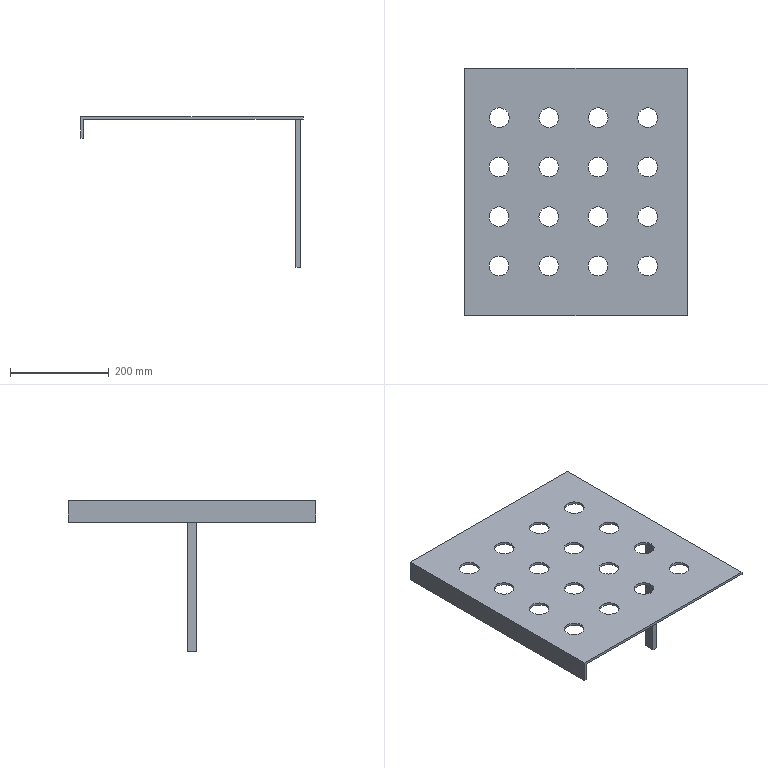Part | SolidWorks | features ICE 3, BaseBody 2 | 1 solid | 45 faces | box 450 x 500 x 305 mm | volume 1181124 mm3 | cylinder 32 | plane 13 | commonest cylinder face diameters 40 x32
STEP:
#1=CARTESIAN_POINT('',(155.,182.201,23.249));
#2=VERTEX_POINT('',#1);
#3=CARTESIAN_POINT('',(195.,182.201,23.249));
#4=VERTEX_POINT('',#3);
#5=CARTESIAN_POINT('',(175.,182.201,23.249));
#6=DIRECTION('',(0.,0.,1.));
#7=DIRECTION('',(1.,0.,0.));
#8=AXIS2_PLACEMENT_3D('',#5,#6,#7);
#9=CIRCLE('',#8,20.);
#10=EDGE_CURVE('',#2,#4,#9,.T.);
#11=ORIENTED_EDGE('',*,*,#10,.F.);
#12=CARTESIAN_POINT('',(155.,182.201,28.249));
#13=VERTEX_POINT('',#12);
#14=CARTESIAN_POINT('',(155.,182.201,23.249));
#15=DIRECTION('',(0.,0.,1.));
#16=VECTOR('',#15,1000.);
#17=LINE('',#14,#16);
#18=EDGE_CURVE('',#2,#13,#17,.T.);
#19=ORIENTED_EDGE('',*,*,#18,.T.);
#20=CARTESIAN_POINT('',(195.,182.201,28.249));
#21=VERTEX_POINT('',#20);
#22=CARTESIAN_POINT('',(175.,182.201,28.249));
#23=DIRECTION('',(0.,0.,1.));
#24=DIRECTION('',(1.,0.,0.));
#25=AXIS2_PLACEMENT_3D('',#22,#23,#24);
#26=CIRCLE('',#25,20.);
#27=EDGE_CURVE('',#13,#21,#26,.T.);
#28=ORIENTED_EDGE('',*,*,#27,.T.);
#29=CARTESIAN_POINT('',(195.,182.201,23.249));
#30=DIRECTION('',(0.,0.,1.));
#31=VECTOR('',#30,1000.);
#32=LINE('',#29,#31);
#33=EDGE_CURVE('',#4,#21,#32,.T.);
#34=ORIENTED_EDGE('',*,*,#33,.F.);
#35=EDGE_LOOP('',(#11,#19,#28,#34));
#36=FACE_OUTER_BOUND('',#35,.T.);
#37=CARTESIAN_POINT('',(175.,182.201,23.249));
#38=DIRECTION('',(0.,0.,1.));
#39=DIRECTION('',(1.,0.,0.));
#40=AXIS2_PLACEMENT_3D('',#37,#38,#39);
#41=CYLINDRICAL_SURFACE('',#40,20.);
#42=ADVANCED_FACE('',(#36),#41,.F.);
#43=CARTESIAN_POINT('',(254.334,182.201,23.249));
#44=VERTEX_POINT('',#43);
#45=CARTESIAN_POINT('',(294.334,182.201,23.249));
#46=VERTEX_POINT('',#45);
#47=CARTESIAN_POINT('',(274.334,182.201,23.249));
#48=DIRECTION('',(0.,0.,1.));
#49=DIRECTION('',(1.,0.,0.));
#50=AXIS2_PLACEMENT_3D('',#47,#48,#49);
#51=CIRCLE('',#50,20.);
#52=EDGE_CURVE('',#44,#46,#51,.T.);
#53=ORIENTED_EDGE('',*,*,#52,.F.);
#54=CARTESIAN_POINT('',(254.334,182.201,28.249));
#55=VERTEX_POINT('',#54);
#56=CARTESIAN_POINT('',(254.334,182.201,23.249));
#57=DIRECTION('',(0.,0.,1.));
#58=VECTOR('',#57,1000.);
#59=LINE('',#56,#58);
#60=EDGE_CURVE('',#44,#55,#59,.T.);
#61=ORIENTED_EDGE('',*,*,#60,.T.);
#62=CARTESIAN_POINT('',(294.334,182.201,28.249));
#63=VERTEX_POINT('',#62);
#64=CARTESIAN_POINT('',(274.334,182.201,28.249));
#65=DIRECTION('',(0.,0.,1.));
#66=DIRECTION('',(1.,0.,0.));
#67=AXIS2_PLACEMENT_3D('',#64,#65,#66);
#68=CIRCLE('',#67,20.);
#69=EDGE_CURVE('',#55,#63,#68,.T.);
#70=ORIENTED_EDGE('',*,*,#69,.T.);
#71=CARTESIAN_POINT('',(294.334,182.201,23.249));
#72=DIRECTION('',(0.,0.,1.));
#73=VECTOR('',#72,1000.);
#74=LINE('',#71,#73);
#75=EDGE_CURVE('',#46,#63,#74,.T.);
#76=ORIENTED_EDGE('',*,*,#75,.F.);
#77=EDGE_LOOP('',(#53,#61,#70,#76));
#78=FACE_OUTER_BOUND('',#77,.T.);
#79=CARTESIAN_POINT('',(274.334,182.201,23.249));
#80=DIRECTION('',(0.,0.,1.));
#81=DIRECTION('',(1.,0.,0.));
#82=AXIS2_PLACEMENT_3D('',#79,#80,#81);
#83=CYLINDRICAL_SURFACE('',#82,20.);
#84=ADVANCED_FACE('',(#78),#83,.F.);
#85=CARTESIAN_POINT('',(355.,182.201,23.249));
#86=VERTEX_POINT('',#85);
#87=CARTESIAN_POINT('',(395.,182.201,23.249));
#88=VERTEX_POINT('',#87);
#89=CARTESIAN_POINT('',(375.,182.201,23.249));
#90=DIRECTION('',(0.,0.,1.));
#91=DIRECTION('',(1.,0.,0.));
#92=AXIS2_PLACEMENT_3D('',#89,#90,#91);
#93=CIRCLE('',#92,20.);
#94=EDGE_CURVE('',#86,#88,#93,.T.);
#95=ORIENTED_EDGE('',*,*,#94,.F.);
#96=CARTESIAN_POINT('',(355.,182.201,28.249));
#97=VERTEX_POINT('',#96);
#98=CARTESIAN_POINT('',(355.,182.201,23.249));
#99=DIRECTION('',(0.,0.,1.));
#100=VECTOR('',#99,1000.);
#101=LINE('',#98,#100);
#102=EDGE_CURVE('',#86,#97,#101,.T.);
#103=ORIENTED_EDGE('',*,*,#102,.T.);
#104=CARTESIAN_POINT('',(395.,182.201,28.249));
#105=VERTEX_POINT('',#104);
#106=CARTESIAN_POINT('',(375.,182.201,28.249));
#107=DIRECTION('',(0.,0.,1.));
#108=DIRECTION('',(1.,0.,0.));
#109=AXIS2_PLACEMENT_3D('',#106,#107,#108);
#110=CIRCLE('',#109,20.);
#111=EDGE_CURVE('',#97,#105,#110,.T.);
#112=ORIENTED_EDGE('',*,*,#111,.T.);
#113=CARTESIAN_POINT('',(395.,182.201,23.249));
#114=DIRECTION('',(0.,0.,1.));
#115=VECTOR('',#114,1000.);
#116=LINE('',#113,#115);
#117=EDGE_CURVE('',#88,#105,#116,.T.);
#118=ORIENTED_EDGE('',*,*,#117,.F.);
#119=EDGE_LOOP('',(#95,#103,#112,#118));
#120=FACE_OUTER_BOUND('',#119,.T.);
#121=CARTESIAN_POINT('',(375.,182.201,23.249));
#122=DIRECTION('',(0.,0.,1.));
#123=DIRECTION('',(1.,0.,0.));
#124=AXIS2_PLACEMENT_3D('',#121,#122,#123);
#125=CYLINDRICAL_SURFACE('',#124,20.);
#126=ADVANCED_FACE('',(#120),#125,.F.);
#127=CARTESIAN_POINT('',(54.334,81.955,23.249));
#128=VERTEX_POINT('',#127);
#129=CARTESIAN_POINT('',(94.334,81.955,23.249));
#130=VERTEX_POINT('',#129);
#131=CARTESIAN_POINT('',(74.334,81.955,23.249));
#132=DIRECTION('',(0.,0.,1.));
#133=DIRECTION('',(1.,0.,0.));
#134=AXIS2_PLACEMENT_3D('',#131,#132,#133);
#135=CIRCLE('',#134,20.);
#136=EDGE_CURVE('',#128,#130,#135,.T.);
#137=ORIENTED_EDGE('',*,*,#136,.F.);
#138=CARTESIAN_POINT('',(54.334,81.955,28.249));
#139=VERTEX_POINT('',#138);
#140=CARTESIAN_POINT('',(54.334,81.955,23.249));
#141=DIRECTION('',(0.,0.,1.));
#142=VECTOR('',#141,1000.);
#143=LINE('',#140,#142);
#144=EDGE_CURVE('',#128,#139,#143,.T.);
#145=ORIENTED_EDGE('',*,*,#144,.T.);
#146=CARTESIAN_POINT('',(94.334,81.955,28.249));
#147=VERTEX_POINT('',#146);
#148=CARTESIAN_POINT('',(74.334,81.955,28.249));
#149=DIRECTION('',(0.,0.,1.));
#150=DIRECTION('',(1.,0.,0.));
#151=AXIS2_PLACEMENT_3D('',#148,#149,#150);
#152=CIRCLE('',#151,20.);
#153=EDGE_CURVE('',#139,#147,#152,.T.);
#154=ORIENTED_EDGE('',*,*,#153,.T.);
#155=CARTESIAN_POINT('',(94.334,81.955,23.249));
#156=DIRECTION('',(0.,0.,1.));
#157=VECTOR('',#156,1000.);
#158=LINE('',#155,#157);
#159=EDGE_CURVE('',#130,#147,#158,.T.);
#160=ORIENTED_EDGE('',*,*,#159,.F.);
#161=EDGE_LOOP('',(#137,#145,#154,#160));
#162=FACE_OUTER_BOUND('',#161,.T.);
#163=CARTESIAN_POINT('',(74.334,81.955,23.249));
#164=DIRECTION('',(0.,0.,1.));
#165=DIRECTION('',(1.,0.,0.));
#166=AXIS2_PLACEMENT_3D('',#163,#164,#165);
#167=CYLINDRICAL_SURFACE('',#166,20.);
#168=ADVANCED_FACE('',(#162),#167,.F.);
#169=CARTESIAN_POINT('',(155.,282.201,23.249));
#170=VERTEX_POINT('',#169);
#171=CARTESIAN_POINT('',(195.,282.201,23.249));
#172=VERTEX_POINT('',#171);
#173=CARTESIAN_POINT('',(175.,282.201,23.249));
#174=DIRECTION('',(0.,0.,1.));
#175=DIRECTION('',(1.,0.,0.));
#176=AXIS2_PLACEMENT_3D('',#173,#174,#175);
#177=CIRCLE('',#176,20.);
#178=EDGE_CURVE('',#170,#172,#177,.T.);
#179=ORIENTED_EDGE('',*,*,#178,.F.);
#180=CARTESIAN_POINT('',(155.,282.201,28.249));
#181=VERTEX_POINT('',#180);
#182=CARTESIAN_POINT('',(155.,282.201,23.249));
#183=DIRECTION('',(0.,0.,1.));
#184=VECTOR('',#183,1000.);
#185=LINE('',#182,#184);
#186=EDGE_CURVE('',#170,#181,#185,.T.);
#187=ORIENTED_EDGE('',*,*,#186,.T.);
#188=CARTESIAN_POINT('',(195.,282.201,28.249));
#189=VERTEX_POINT('',#188);
#190=CARTESIAN_POINT('',(175.,282.201,28.249));
#191=DIRECTION('',(0.,0.,1.));
#192=DIRECTION('',(1.,0.,0.));
#193=AXIS2_PLACEMENT_3D('',#190,#191,#192);
#194=CIRCLE('',#193,20.);
#195=EDGE_CURVE('',#181,#189,#194,.T.);
#196=ORIENTED_EDGE('',*,*,#195,.T.);
#197=CARTESIAN_POINT('',(195.,282.201,23.249));
#198=DIRECTION('',(0.,0.,1.));
#199=VECTOR('',#198,1000.);
#200=LINE('',#197,#199);
#201=EDGE_CURVE('',#172,#189,#200,.T.);
#202=ORIENTED_EDGE('',*,*,#201,.F.);
#203=EDGE_LOOP('',(#179,#187,#196,#202));
#204=FACE_OUTER_BOUND('',#203,.T.);
#205=CARTESIAN_POINT('',(175.,282.201,23.249));
#206=DIRECTION('',(0.,0.,1.));
#207=DIRECTION('',(1.,0.,0.));
#208=AXIS2_PLACEMENT_3D('',#205,#206,#207);
#209=CYLINDRICAL_SURFACE('',#208,20.);
#210=ADVANCED_FACE('',(#204),#209,.F.);
#211=CARTESIAN_POINT('',(255.,282.201,23.249));
#212=VERTEX_POINT('',#211);
#213=CARTESIAN_POINT('',(295.,282.201,23.249));
#214=VERTEX_POINT('',#213);
#215=CARTESIAN_POINT('',(275.,282.201,23.249));
#216=DIRECTION('',(0.,0.,1.));
#217=DIRECTION('',(1.,0.,0.));
#218=AXIS2_PLACEMENT_3D('',#215,#216,#217);
#219=CIRCLE('',#218,20.);
#220=EDGE_CURVE('',#212,#214,#219,.T.);
#221=ORIENTED_EDGE('',*,*,#220,.F.);
#222=CARTESIAN_POINT('',(255.,282.201,28.249));
#223=VERTEX_POINT('',#222);
#224=CARTESIAN_POINT('',(255.,282.201,23.249));
#225=DIRECTION('',(0.,0.,1.));
#226=VECTOR('',#225,1000.);
#227=LINE('',#224,#226);
#228=EDGE_CURVE('',#212,#223,#227,.T.);
#229=ORIENTED_EDGE('',*,*,#228,.T.);
#230=CARTESIAN_POINT('',(295.,282.201,28.249));
#231=VERTEX_POINT('',#230);
#232=CARTESIAN_POINT('',(275.,282.201,28.249));
#233=DIRECTION('',(0.,0.,1.));
#234=DIRECTION('',(1.,0.,0.));
#235=AXIS2_PLACEMENT_3D('',#232,#233,#234);
#236=CIRCLE('',#235,20.);
#237=EDGE_CURVE('',#223,#231,#236,.T.);
#238=ORIENTED_EDGE('',*,*,#237,.T.);
#239=CARTESIAN_POINT('',(295.,282.201,23.249));
#240=DIRECTION('',(0.,0.,1.));
#241=VECTOR('',#240,1000.);
#242=LINE('',#239,#241);
#243=EDGE_CURVE('',#214,#231,#242,.T.);
#244=ORIENTED_EDGE('',*,*,#243,.F.);
#245=EDGE_LOOP('',(#221,#229,#238,#244));
#246=FACE_OUTER_BOUND('',#245,.T.);
#247=CARTESIAN_POINT('',(275.,282.201,23.249));
#248=DIRECTION('',(0.,0.,1.));
#249=DIRECTION('',(1.,0.,0.));
#250=AXIS2_PLACEMENT_3D('',#247,#248,#249);
#251=CYLINDRICAL_SURFACE('',#250,20.);
#252=ADVANCED_FACE('',(#246),#251,.F.);
#253=CARTESIAN_POINT('',(355.,282.201,23.249));
#254=VERTEX_POINT('',#253);
#255=CARTESIAN_POINT('',(395.,282.201,23.249));
#256=VERTEX_POINT('',#255);
#257=CARTESIAN_POINT('',(375.,282.201,23.249));
#258=DIRECTION('',(0.,0.,1.));
#259=DIRECTION('',(1.,0.,0.));
#260=AXIS2_PLACEMENT_3D('',#257,#258,#259);
#261=CIRCLE('',#260,20.);
#262=EDGE_CURVE('',#254,#256,#261,.T.);
#263=ORIENTED_EDGE('',*,*,#262,.F.);
#264=CARTESIAN_POINT('',(355.,282.201,28.249));
#265=VERTEX_POINT('',#264);
#266=CARTESIAN_POINT('',(355.,282.201,23.249));
#267=DIRECTION('',(0.,0.,1.));
#268=VECTOR('',#267,1000.);
#269=LINE('',#266,#268);
#270=EDGE_CURVE('',#254,#265,#269,.T.);
#271=ORIENTED_EDGE('',*,*,#270,.T.);
#272=CARTESIAN_POINT('',(395.,282.201,28.249));
#273=VERTEX_POINT('',#272);
#274=CARTESIAN_POINT('',(375.,282.201,28.249));
#275=DIRECTION('',(0.,0.,1.));
#276=DIRECTION('',(1.,0.,0.));
#277=AXIS2_PLACEMENT_3D('',#274,#275,#276);
#278=CIRCLE('',#277,20.);
#279=EDGE_CURVE('',#265,#273,#278,.T.);
#280=ORIENTED_EDGE('',*,*,#279,.T.);
#281=CARTESIAN_POINT('',(395.,282.201,23.249));
#282=DIRECTION('',(0.,0.,1.));
#283=VECTOR('',#282,1000.);
#284=LINE('',#281,#283);
#285=EDGE_CURVE('',#256,#273,#284,.T.);
#286=ORIENTED_EDGE('',*,*,#285,.F.);
#287=EDGE_LOOP('',(#263,#271,#280,#286));
#288=FACE_OUTER_BOUND('',#287,.T.);
#289=CARTESIAN_POINT('',(375.,282.201,23.249));
#290=DIRECTION('',(0.,0.,1.));
#291=DIRECTION('',(1.,0.,0.));
#292=AXIS2_PLACEMENT_3D('',#289,#290,#291);
#293=CYLINDRICAL_SURFACE('',#292,20.);
#294=ADVANCED_FACE('',(#288),#293,.F.);
#295=CARTESIAN_POINT('',(54.334,182.201,23.249));
#296=VERTEX_POINT('',#295);
#297=CARTESIAN_POINT('',(94.334,182.201,23.249));
#298=VERTEX_POINT('',#297);
#299=CARTESIAN_POINT('',(74.334,182.201,23.249));
#300=DIRECTION('',(0.,0.,1.));
#301=DIRECTION('',(1.,0.,0.));
#302=AXIS2_PLACEMENT_3D('',#299,#300,#301);
#303=CIRCLE('',#302,20.);
#304=EDGE_CURVE('',#296,#298,#303,.T.);
#305=ORIENTED_EDGE('',*,*,#304,.F.);
#306=CARTESIAN_POINT('',(54.334,182.201,28.249));
#307=VERTEX_POINT('',#306);
#308=CARTESIAN_POINT('',(54.334,182.201,23.249));
#309=DIRECTION('',(0.,0.,1.));
#310=VECTOR('',#309,1000.);
#311=LINE('',#308,#310);
#312=EDGE_CURVE('',#296,#307,#311,.T.);
#313=ORIENTED_EDGE('',*,*,#312,.T.);
#314=CARTESIAN_POINT('',(94.334,182.201,28.249));
#315=VERTEX_POINT('',#314);
#316=CARTESIAN_POINT('',(74.334,182.201,28.249));
#317=DIRECTION('',(0.,0.,1.));
#318=DIRECTION('',(1.,0.,0.));
#319=AXIS2_PLACEMENT_3D('',#316,#317,#318);
#320=CIRCLE('',#319,20.);
#321=EDGE_CURVE('',#307,#315,#320,.T.);
#322=ORIENTED_EDGE('',*,*,#321,.T.);
#323=CARTESIAN_POINT('',(94.334,182.201,23.249));
#324=DIRECTION('',(0.,0.,1.));
#325=VECTOR('',#324,1000.);
#326=LINE('',#323,#325);
#327=EDGE_CURVE('',#298,#315,#326,.T.);
#328=ORIENTED_EDGE('',*,*,#327,.F.);
#329=EDGE_LOOP('',(#305,#313,#322,#328));
#330=FACE_OUTER_BOUND('',#329,.T.);
#331=CARTESIAN_POINT('',(74.334,182.201,23.249));
#332=DIRECTION('',(0.,0.,1.));
#333=DIRECTION('',(1.,0.,0.));
#334=AXIS2_PLACEMENT_3D('',#331,#332,#333);
#335=CYLINDRICAL_SURFACE('',#334,20.);
#336=ADVANCED_FACE('',(#330),#335,.F.);
#337=CARTESIAN_POINT('',(355.,-18.045,23.249));
#338=VERTEX_POINT('',#337);
#339=CARTESIAN_POINT('',(395.,-18.045,23.249));
#340=VERTEX_POINT('',#339);
#341=CARTESIAN_POINT('',(375.,-18.045,23.249));
#342=DIRECTION('',(0.,0.,1.));
#343=DIRECTION('',(1.,0.,0.));
#344=AXIS2_PLACEMENT_3D('',#341,#342,#343);
#345=CIRCLE('',#344,20.);
#346=EDGE_CURVE('',#338,#340,#345,.T.);
#347=ORIENTED_EDGE('',*,*,#346,.F.);
#348=CARTESIAN_POINT('',(355.,-18.045,28.249));
#349=VERTEX_POINT('',#348);
#350=CARTESIAN_POINT('',(355.,-18.045,23.249));
#351=DIRECTION('',(0.,0.,1.));
#352=VECTOR('',#351,1000.);
#353=LINE('',#350,#352);
#354=EDGE_CURVE('',#338,#349,#353,.T.);
#355=ORIENTED_EDGE('',*,*,#354,.T.);
#356=CARTESIAN_POINT('',(395.,-18.045,28.249));
#357=VERTEX_POINT('',#356);
#358=CARTESIAN_POINT('',(375.,-18.045,28.249));
#359=DIRECTION('',(0.,0.,1.));
#360=DIRECTION('',(1.,0.,0.));
#361=AXIS2_PLACEMENT_3D('',#358,#359,#360);
#362=CIRCLE('',#361,20.);
#363=EDGE_CURVE('',#349,#357,#362,.T.);
#364=ORIENTED_EDGE('',*,*,#363,.T.);
#365=CARTESIAN_POINT('',(395.,-18.045,23.249));
#366=DIRECTION('',(0.,0.,1.));
#367=VECTOR('',#366,1000.);
#368=LINE('',#365,#367);
#369=EDGE_CURVE('',#340,#357,#368,.T.);
#370=ORIENTED_EDGE('',*,*,#369,.F.);
#371=EDGE_LOOP('',(#347,#355,#364,#370));
#372=FACE_OUTER_BOUND('',#371,.T.);
#373=CARTESIAN_POINT('',(375.,-18.045,23.249));
#374=DIRECTION('',(0.,0.,1.));
#375=DIRECTION('',(1.,0.,0.));
#376=AXIS2_PLACEMENT_3D('',#373,#374,#375);
#377=CYLINDRICAL_SURFACE('',#376,20.);
#378=ADVANCED_FACE('',(#372),#377,.F.);
#379=CARTESIAN_POINT('',(254.334,-18.045,23.249));
#380=VERTEX_POINT('',#379);
#381=CARTESIAN_POINT('',(294.334,-18.045,23.249));
#382=VERTEX_POINT('',#381);
#383=CARTESIAN_POINT('',(274.334,-18.045,23.249));
#384=DIRECTION('',(0.,0.,1.));
#385=DIRECTION('',(1.,0.,0.));
#386=AXIS2_PLACEMENT_3D('',#383,#384,#385);
#387=CIRCLE('',#386,20.);
#388=EDGE_CURVE('',#380,#382,#387,.T.);
#389=ORIENTED_EDGE('',*,*,#388,.F.);
#390=CARTESIAN_POINT('',(254.334,-18.045,28.249));
#391=VERTEX_POINT('',#390);
#392=CARTESIAN_POINT('',(254.334,-18.045,23.249));
#393=DIRECTION('',(0.,0.,1.));
#394=VECTOR('',#393,1000.);
#395=LINE('',#392,#394);
#396=EDGE_CURVE('',#380,#391,#395,.T.);
#397=ORIENTED_EDGE('',*,*,#396,.T.);
#398=CARTESIAN_POINT('',(294.334,-18.045,28.249));
#399=VERTEX_POINT('',#398);
#400=CARTESIAN_POINT('',(274.334,-18.045,28.249));
#401=DIRECTION('',(0.,0.,1.));
#402=DIRECTION('',(1.,0.,0.));
#403=AXIS2_PLACEMENT_3D('',#400,#401,#402);
#404=CIRCLE('',#403,20.);
#405=EDGE_CURVE('',#391,#399,#404,.T.);
#406=ORIENTED_EDGE('',*,*,#405,.T.);
#407=CARTESIAN_POINT('',(294.334,-18.045,23.249));
#408=DIRECTION('',(0.,0.,1.));
#409=VECTOR('',#408,1000.);
#410=LINE('',#407,#409);
#411=EDGE_CURVE('',#382,#399,#410,.T.);
#412=ORIENTED_EDGE('',*,*,#411,.F.);
#413=EDGE_LOOP('',(#389,#397,#406,#412));
#414=FACE_OUTER_BOUND('',#413,.T.);
#415=CARTESIAN_POINT('',(274.334,-18.045,23.249));
#416=DIRECTION('',(0.,0.,1.));
#417=DIRECTION('',(1.,0.,0.));
#418=AXIS2_PLACEMENT_3D('',#415,#416,#417);
#419=CYLINDRICAL_SURFACE('',#418,20.);
#420=ADVANCED_FACE('',(#414),#419,.F.);
#421=CARTESIAN_POINT('',(155.,-18.045,23.249));
#422=VERTEX_POINT('',#421);
#423=CARTESIAN_POINT('',(195.,-18.045,23.249));
#424=VERTEX_POINT('',#423);
#425=CARTESIAN_POINT('',(175.,-18.045,23.249));
#426=DIRECTION('',(0.,0.,1.));
#427=DIRECTION('',(1.,0.,0.));
#428=AXIS2_PLACEMENT_3D('',#425,#426,#427);
#429=CIRCLE('',#428,20.);
#430=EDGE_CURVE('',#422,#424,#429,.T.);
#431=ORIENTED_EDGE('',*,*,#430,.F.);
#432=CARTESIAN_POINT('',(155.,-18.045,28.249));
#433=VERTEX_POINT('',#432);
#434=CARTESIAN_POINT('',(155.,-18.045,23.249));
#435=DIRECTION('',(0.,0.,1.));
#436=VECTOR('',#435,1000.);
#437=LINE('',#434,#436);
#438=EDGE_CURVE('',#422,#433,#437,.T.);
#439=ORIENTED_EDGE('',*,*,#438,.T.);
#440=CARTESIAN_POINT('',(195.,-18.045,28.249));
#441=VERTEX_POINT('',#440);
#442=CARTESIAN_POINT('',(175.,-18.045,28.249));
#443=DIRECTION('',(0.,0.,1.));
#444=DIRECTION('',(1.,0.,0.));
#445=AXIS2_PLACEMENT_3D('',#442,#443,#444);
#446=CIRCLE('',#445,20.);
#447=EDGE_CURVE('',#433,#441,#446,.T.);
#448=ORIENTED_EDGE('',*,*,#447,.T.);
#449=CARTESIAN_POINT('',(195.,-18.045,23.249));
#450=DIRECTION('',(0.,0.,1.));
#451=VECTOR('',#450,1000.);
#452=LINE('',#449,#451);
#453=EDGE_CURVE('',#424,#441,#452,.T.);
#454=ORIENTED_EDGE('',*,*,#453,.F.);
#455=EDGE_LOOP('',(#431,#439,#448,#454));
#456=FACE_OUTER_BOUND('',#455,.T.);
#457=CARTESIAN_POINT('',(175.,-18.045,23.249));
#458=DIRECTION('',(0.,0.,1.));
#459=DIRECTION('',(1.,0.,0.));
#460=AXIS2_PLACEMENT_3D('',#457,#458,#459);
#461=CYLINDRICAL_SURFACE('',#460,20.);
#462=ADVANCED_FACE('',(#456),#461,.F.);
#463=CARTESIAN_POINT('',(155.,81.955,23.249));
#464=VERTEX_POINT('',#463);
#465=CARTESIAN_POINT('',(195.,81.955,23.249));
#466=VERTEX_POINT('',#465);
#467=CARTESIAN_POINT('',(175.,81.955,23.249));
#468=DIRECTION('',(0.,0.,1.));
#469=DIRECTION('',(1.,0.,0.));
#470=AXIS2_PLACEMENT_3D('',#467,#468,#469);
#471=CIRCLE('',#470,20.);
#472=EDGE_CURVE('',#464,#466,#471,.T.);
#473=ORIENTED_EDGE('',*,*,#472,.F.);
#474=CARTESIAN_POINT('',(155.,81.955,28.249));
#475=VERTEX_POINT('',#474);
#476=CARTESIAN_POINT('',(155.,81.955,23.249));
#477=DIRECTION('',(0.,0.,1.));
#478=VECTOR('',#477,1000.);
#479=LINE('',#476,#478);
#480=EDGE_CURVE('',#464,#475,#479,.T.);
#481=ORIENTED_EDGE('',*,*,#480,.T.);
#482=CARTESIAN_POINT('',(195.,81.955,28.249));
#483=VERTEX_POINT('',#482);
#484=CARTESIAN_POINT('',(175.,81.955,28.249));
#485=DIRECTION('',(0.,0.,1.));
#486=DIRECTION('',(1.,0.,0.));
#487=AXIS2_PLACEMENT_3D('',#484,#485,#486);
#488=CIRCLE('',#487,20.);
#489=EDGE_CURVE('',#475,#483,#488,.T.);
#490=ORIENTED_EDGE('',*,*,#489,.T.);
#491=CARTESIAN_POINT('',(195.,81.955,23.249));
#492=DIRECTION('',(0.,0.,1.));
#493=VECTOR('',#492,1000.);
#494=LINE('',#491,#493);
#495=EDGE_CURVE('',#466,#483,#494,.T.);
#496=ORIENTED_EDGE('',*,*,#495,.F.);
#497=EDGE_LOOP('',(#473,#481,#490,#496));
#498=FACE_OUTER_BOUND('',#497,.T.);
#499=CARTESIAN_POINT('',(175.,81.955,23.249));
#500=DIRECTION('',(0.,0.,1.));
#501=DIRECTION('',(1.,0.,0.));
#502=AXIS2_PLACEMENT_3D('',#499,#500,#501);
#503=CYLINDRICAL_SURFACE('',#502,20.);
#504=ADVANCED_FACE('',(#498),#503,.F.);
#505=CARTESIAN_POINT('',(254.334,81.955,23.249));
#506=VERTEX_POINT('',#505);
#507=CARTESIAN_POINT('',(294.334,81.955,23.249));
#508=VERTEX_POINT('',#507);
#509=CARTESIAN_POINT('',(274.334,81.955,23.249));
#510=DIRECTION('',(0.,0.,1.));
#511=DIRECTION('',(1.,0.,0.));
#512=AXIS2_PLACEMENT_3D('',#509,#510,#511);
#513=CIRCLE('',#512,20.);
#514=EDGE_CURVE('',#506,#508,#513,.T.);
#515=ORIENTED_EDGE('',*,*,#514,.F.);
#516=CARTESIAN_POINT('',(254.334,81.955,28.249));
#517=VERTEX_POINT('',#516);
#518=CARTESIAN_POINT('',(254.334,81.955,23.249));
#519=DIRECTION('',(0.,0.,1.));
#520=VECTOR('',#519,1000.);
#521=LINE('',#518,#520);
#522=EDGE_CURVE('',#506,#517,#521,.T.);
#523=ORIENTED_EDGE('',*,*,#522,.T.);
#524=CARTESIAN_POINT('',(294.334,81.955,28.249));
#525=VERTEX_POINT('',#524);
#526=CARTESIAN_POINT('',(274.334,81.955,28.249));
#527=DIRECTION('',(0.,0.,1.));
#528=DIRECTION('',(1.,0.,0.));
#529=AXIS2_PLACEMENT_3D('',#526,#527,#528);
#530=CIRCLE('',#529,20.);
#531=EDGE_CURVE('',#517,#525,#530,.T.);
#532=ORIENTED_EDGE('',*,*,#531,.T.);
#533=CARTESIAN_POINT('',(294.334,81.955,23.249));
#534=DIRECTION('',(0.,0.,1.));
#535=VECTOR('',#534,1000.);
#536=LINE('',#533,#535);
#537=EDGE_CURVE('',#508,#525,#536,.T.);
#538=ORIENTED_EDGE('',*,*,#537,.F.);
#539=EDGE_LOOP('',(#515,#523,#532,#538));
#540=FACE_OUTER_BOUND('',#539,.T.);
#541=CARTESIAN_POINT('',(274.334,81.955,23.249));
#542=DIRECTION('',(0.,0.,1.));
#543=DIRECTION('',(1.,0.,0.));
#544=AXIS2_PLACEMENT_3D('',#541,#542,#543);
#545=CYLINDRICAL_SURFACE('',#544,20.);
#546=ADVANCED_FACE('',(#540),#545,.F.);
#547=CARTESIAN_POINT('',(355.,81.955,23.249));
#548=VERTEX_POINT('',#547);
#549=CARTESIAN_POINT('',(395.,81.955,23.249));
#550=VERTEX_POINT('',#549);
#551=CARTESIAN_POINT('',(375.,81.955,23.249));
#552=DIRECTION('',(0.,0.,1.));
#553=DIRECTION('',(1.,0.,0.));
#554=AXIS2_PLACEMENT_3D('',#551,#552,#553);
#555=CIRCLE('',#554,20.);
#556=EDGE_CURVE('',#548,#550,#555,.T.);
#557=ORIENTED_EDGE('',*,*,#556,.F.);
#558=CARTESIAN_POINT('',(355.,81.955,28.249));
#559=VERTEX_POINT('',#558);
#560=CARTESIAN_POINT('',(355.,81.955,23.249));
#561=DIRECTION('',(0.,0.,1.));
#562=VECTOR('',#561,1000.);
#563=LINE('',#560,#562);
#564=EDGE_CURVE('',#548,#559,#563,.T.);
#565=ORIENTED_EDGE('',*,*,#564,.T.);
#566=CARTESIAN_POINT('',(395.,81.955,28.249));
#567=VERTEX_POINT('',#566);
#568=CARTESIAN_POINT('',(375.,81.955,28.249));
#569=DIRECTION('',(0.,0.,1.));
#570=DIRECTION('',(1.,0.,0.));
#571=AXIS2_PLACEMENT_3D('',#568,#569,#570);
#572=CIRCLE('',#571,20.);
#573=EDGE_CURVE('',#559,#567,#572,.T.);
#574=ORIENTED_EDGE('',*,*,#573,.T.);
#575=CARTESIAN_POINT('',(395.,81.955,23.249));
#576=DIRECTION('',(0.,0.,1.));
#577=VECTOR('',#576,1000.);
#578=LINE('',#575,#577);
#579=EDGE_CURVE('',#550,#567,#578,.T.);
#580=ORIENTED_EDGE('',*,*,#579,.F.);
#581=EDGE_LOOP('',(#557,#565,#574,#580));
#582=FACE_OUTER_BOUND('',#581,.T.);
#583=CARTESIAN_POINT('',(375.,81.955,23.249));
#584=DIRECTION('',(0.,0.,1.));
#585=DIRECTION('',(1.,0.,0.));
#586=AXIS2_PLACEMENT_3D('',#583,#584,#585);
#587=CYLINDRICAL_SURFACE('',#586,20.);
#588=ADVANCED_FACE('',(#582),#587,.F.);
#589=CARTESIAN_POINT('',(54.334,-18.045,23.249));
#590=VERTEX_POINT('',#589);
#591=CARTESIAN_POINT('',(94.334,-18.045,23.249));
#592=VERTEX_POINT('',#591);
#593=CARTESIAN_POINT('',(74.334,-18.045,23.249));
#594=DIRECTION('',(0.,0.,1.));
#595=DIRECTION('',(1.,0.,0.));
#596=AXIS2_PLACEMENT_3D('',#593,#594,#595);
#597=CIRCLE('',#596,20.);
#598=EDGE_CURVE('',#590,#592,#597,.T.);
#599=ORIENTED_EDGE('',*,*,#598,.F.);
#600=CARTESIAN_POINT('',(54.334,-18.045,28.249));
#601=VERTEX_POINT('',#600);
#602=CARTESIAN_POINT('',(54.334,-18.045,23.249));
#603=DIRECTION('',(0.,0.,1.));
#604=VECTOR('',#603,1000.);
#605=LINE('',#602,#604);
#606=EDGE_CURVE('',#590,#601,#605,.T.);
#607=ORIENTED_EDGE('',*,*,#606,.T.);
#608=CARTESIAN_POINT('',(94.334,-18.045,28.249));
#609=VERTEX_POINT('',#608);
#610=CARTESIAN_POINT('',(74.334,-18.045,28.249));
#611=DIRECTION('',(0.,0.,1.));
#612=DIRECTION('',(1.,0.,0.));
#613=AXIS2_PLACEMENT_3D('',#610,#611,#612);
#614=CIRCLE('',#613,20.);
#615=EDGE_CURVE('',#601,#609,#614,.T.);
#616=ORIENTED_EDGE('',*,*,#615,.T.);
#617=CARTESIAN_POINT('',(94.334,-18.045,23.249));
#618=DIRECTION('',(0.,0.,1.));
#619=VECTOR('',#618,1000.);
#620=LINE('',#617,#619);
#621=EDGE_CURVE('',#592,#609,#620,.T.);
#622=ORIENTED_EDGE('',*,*,#621,.F.);
#623=EDGE_LOOP('',(#599,#607,#616,#622));
#624=FACE_OUTER_BOUND('',#623,.T.);
#625=CARTESIAN_POINT('',(74.334,-18.045,23.249));
#626=DIRECTION('',(0.,0.,1.));
#627=DIRECTION('',(1.,0.,0.));
#628=AXIS2_PLACEMENT_3D('',#625,#626,#627);
#629=CYLINDRICAL_SURFACE('',#628,20.);
#630=ADVANCED_FACE('',(#624),#629,.F.);
#631=CARTESIAN_POINT('',(55.,282.201,23.249));
#632=VERTEX_POINT('',#631);
#633=CARTESIAN_POINT('',(95.,282.201,23.249));
#634=VERTEX_POINT('',#633);
#635=CARTESIAN_POINT('',(75.,282.201,23.249));
#636=DIRECTION('',(0.,0.,1.));
#637=DIRECTION('',(1.,0.,0.));
#638=AXIS2_PLACEMENT_3D('',#635,#636,#637);
#639=CIRCLE('',#638,20.);
#640=EDGE_CURVE('',#632,#634,#639,.T.);
#641=ORIENTED_EDGE('',*,*,#640,.F.);
#642=CARTESIAN_POINT('',(55.,282.201,28.249));
#643=VERTEX_POINT('',#642);
#644=CARTESIAN_POINT('',(55.,282.201,23.249));
#645=DIRECTION('',(0.,0.,1.));
#646=VECTOR('',#645,1000.);
#647=LINE('',#644,#646);
#648=EDGE_CURVE('',#632,#643,#647,.T.);
#649=ORIENTED_EDGE('',*,*,#648,.T.);
#650=CARTESIAN_POINT('',(95.,282.201,28.249));
#651=VERTEX_POINT('',#650);
#652=CARTESIAN_POINT('',(75.,282.201,28.249));
#653=DIRECTION('',(0.,0.,1.));
#654=DIRECTION('',(1.,0.,0.));
#655=AXIS2_PLACEMENT_3D('',#652,#653,#654);
#656=CIRCLE('',#655,20.);
#657=EDGE_CURVE('',#643,#651,#656,.T.);
#658=ORIENTED_EDGE('',*,*,#657,.T.);
#659=CARTESIAN_POINT('',(95.,282.201,23.249));
#660=DIRECTION('',(0.,0.,1.));
#661=VECTOR('',#660,1000.);
#662=LINE('',#659,#661);
#663=EDGE_CURVE('',#634,#651,#662,.T.);
#664=ORIENTED_EDGE('',*,*,#663,.F.);
#665=EDGE_LOOP('',(#641,#649,#658,#664));
#666=FACE_OUTER_BOUND('',#665,.T.);
#667=CARTESIAN_POINT('',(75.,282.201,23.249));
#668=DIRECTION('',(0.,0.,1.));
#669=DIRECTION('',(1.,0.,0.));
#670=AXIS2_PLACEMENT_3D('',#667,#668,#669);
#671=CYLINDRICAL_SURFACE('',#670,20.);
#672=ADVANCED_FACE('',(#666),#671,.F.);
#673=CARTESIAN_POINT('',(450.,121.955,23.249));
#674=VERTEX_POINT('',#673);
#675=CARTESIAN_POINT('',(450.,141.955,23.249));
#676=VERTEX_POINT('',#675);
#677=CARTESIAN_POINT('',(450.,381.955,23.249));
#678=DIRECTION('',(0.,1.,0.));
#679=VECTOR('',#678,1000.);
#680=LINE('',#677,#679);
#681=EDGE_CURVE('',#674,#676,#680,.T.);
#682=ORIENTED_EDGE('',*,*,#681,.F.);
#683=CARTESIAN_POINT('',(450.,121.955,-276.751));
#684=VERTEX_POINT('',#683);
#685=CARTESIAN_POINT('',(450.,121.955,-276.751));
#686=DIRECTION('',(0.,0.,1.));
#687=VECTOR('',#686,1000.);
#688=LINE('',#685,#687);
#689=EDGE_CURVE('',#684,#674,#688,.T.);
#690=ORIENTED_EDGE('',*,*,#689,.F.);
#691=CARTESIAN_POINT('',(450.,141.955,-276.751));
#692=VERTEX_POINT('',#691);
#693=CARTESIAN_POINT('',(450.,141.955,-276.751));
#694=DIRECTION('',(0.,-1.,0.));
#695=VECTOR('',#694,1000.);
#696=LINE('',#693,#695);
#697=EDGE_CURVE('',#692,#684,#696,.T.);
#698=ORIENTED_EDGE('',*,*,#697,.F.);
#699=CARTESIAN_POINT('',(450.,141.955,-276.751));
#700=DIRECTION('',(0.,0.,1.));
#701=VECTOR('',#700,1000.);
#702=LINE('',#699,#701);
#703=EDGE_CURVE('',#692,#676,#702,.T.);
#704=ORIENTED_EDGE('',*,*,#703,.T.);
#705=EDGE_LOOP('',(#682,#690,#698,#704));
#706=FACE_OUTER_BOUND('',#705,.T.);
#707=CARTESIAN_POINT('',(450.,131.955,-276.751));
#708=DIRECTION('',(-1.,0.,0.));
#709=DIRECTION('',(0.,0.,1.));
#710=AXIS2_PLACEMENT_3D('',#707,#708,#709);
#711=PLANE('',#710);
#712=ADVANCED_FACE('',(#706),#711,.F.);
#713=CARTESIAN_POINT('',(440.,121.955,23.249));
#714=VERTEX_POINT('',#713);
#715=CARTESIAN_POINT('',(440.,141.955,23.249));
#716=VERTEX_POINT('',#715);
#717=CARTESIAN_POINT('',(440.,121.955,23.249));
#718=DIRECTION('',(0.,1.,0.));
#719=VECTOR('',#718,1000.);
#720=LINE('',#717,#719);
#721=EDGE_CURVE('',#714,#716,#720,.T.);
#722=ORIENTED_EDGE('',*,*,#721,.T.);
#723=CARTESIAN_POINT('',(440.,141.955,-276.751));
#724=VERTEX_POINT('',#723);
#725=CARTESIAN_POINT('',(440.,141.955,-276.751));
#726=DIRECTION('',(0.,0.,1.));
#727=VECTOR('',#726,1000.);
#728=LINE('',#725,#727);
#729=EDGE_CURVE('',#724,#716,#728,.T.);
#730=ORIENTED_EDGE('',*,*,#729,.F.);
#731=CARTESIAN_POINT('',(440.,121.955,-276.751));
#732=VERTEX_POINT('',#731);
#733=CARTESIAN_POINT('',(440.,121.955,-276.751));
#734=DIRECTION('',(0.,1.,0.));
#735=VECTOR('',#734,1000.);
#736=LINE('',#733,#735);
#737=EDGE_CURVE('',#732,#724,#736,.T.);
#738=ORIENTED_EDGE('',*,*,#737,.F.);
#739=CARTESIAN_POINT('',(440.,121.955,-276.751));
#740=DIRECTION('',(0.,0.,1.));
#741=VECTOR('',#740,1000.);
#742=LINE('',#739,#741);
#743=EDGE_CURVE('',#732,#714,#742,.T.);
#744=ORIENTED_EDGE('',*,*,#743,.T.);
#745=EDGE_LOOP('',(#722,#730,#738,#744));
#746=FACE_OUTER_BOUND('',#745,.T.);
#747=CARTESIAN_POINT('',(440.,121.955,-276.751));
#748=DIRECTION('',(1.,0.,0.));
#749=DIRECTION('',(0.,0.,-1.));
#750=AXIS2_PLACEMENT_3D('',#747,#748,#749);
#751=PLANE('',#750);
#752=ADVANCED_FACE('',(#746),#751,.F.);
#753=CARTESIAN_POINT('',(440.,141.955,23.249));
#754=DIRECTION('',(1.,0.,0.));
#755=VECTOR('',#754,1000.);
#756=LINE('',#753,#755);
#757=EDGE_CURVE('',#716,#676,#756,.T.);
#758=ORIENTED_EDGE('',*,*,#757,.T.);
#759=ORIENTED_EDGE('',*,*,#703,.F.);
#760=CARTESIAN_POINT('',(440.,141.955,-276.751));
#761=DIRECTION('',(1.,0.,0.));
#762=VECTOR('',#761,1000.);
#763=LINE('',#760,#762);
#764=EDGE_CURVE('',#724,#692,#763,.T.);
#765=ORIENTED_EDGE('',*,*,#764,.F.);
#766=ORIENTED_EDGE('',*,*,#729,.T.);
#767=EDGE_LOOP('',(#758,#759,#765,#766));
#768=FACE_OUTER_BOUND('',#767,.T.);
#769=CARTESIAN_POINT('',(440.,141.955,-276.751));
#770=DIRECTION('',(0.,-1.,0.));
#771=DIRECTION('',(0.,0.,-1.));
#772=AXIS2_PLACEMENT_3D('',#769,#770,#771);
#773=PLANE('',#772);
#774=ADVANCED_FACE('',(#768),#773,.F.);
#775=CARTESIAN_POINT('',(450.,121.955,23.249));
#776=DIRECTION('',(-1.,0.,0.));
#777=VECTOR('',#776,1000.);
#778=LINE('',#775,#777);
#779=EDGE_CURVE('',#674,#714,#778,.T.);
#780=ORIENTED_EDGE('',*,*,#779,.T.);
#781=ORIENTED_EDGE('',*,*,#743,.F.);
#782=CARTESIAN_POINT('',(450.,121.955,-276.751));
#783=DIRECTION('',(-1.,0.,0.));
#784=VECTOR('',#783,1000.);
#785=LINE('',#782,#784);
#786=EDGE_CURVE('',#684,#732,#785,.T.);
#787=ORIENTED_EDGE('',*,*,#786,.F.);
#788=ORIENTED_EDGE('',*,*,#689,.T.);
#789=EDGE_LOOP('',(#780,#781,#787,#788));
#790=FACE_OUTER_BOUND('',#789,.T.);
#791=CARTESIAN_POINT('',(450.,121.955,-276.751));
#792=DIRECTION('',(0.,1.,0.));
#793=DIRECTION('',(0.,0.,1.));
#794=AXIS2_PLACEMENT_3D('',#791,#792,#793);
#795=PLANE('',#794);
#796=ADVANCED_FACE('',(#790),#795,.F.);
#797=ORIENTED_EDGE('',*,*,#737,.T.);
#798=ORIENTED_EDGE('',*,*,#764,.T.);
#799=ORIENTED_EDGE('',*,*,#697,.T.);
#800=ORIENTED_EDGE('',*,*,#786,.T.);
#801=EDGE_LOOP('',(#797,#798,#799,#800));
#802=FACE_OUTER_BOUND('',#801,.T.);
#803=CARTESIAN_POINT('',(0.,0.,-276.751));
#804=DIRECTION('',(0.,0.,-1.));
#805=DIRECTION('',(-1.,0.,0.));
#806=AXIS2_PLACEMENT_3D('',#803,#804,#805);
#807=PLANE('',#806);
#808=ADVANCED_FACE('',(#802),#807,.T.);
#809=ORIENTED_EDGE('',*,*,#779,.F.);
#810=ORIENTED_EDGE('',*,*,#681,.T.);
#811=ORIENTED_EDGE('',*,*,#757,.F.);
#812=ORIENTED_EDGE('',*,*,#721,.F.);
#813=EDGE_LOOP('',(#809,#810,#811,#812));
#814=FACE_BOUND('',#813,.T.);
#815=CARTESIAN_POINT('',(274.334,81.955,23.249));
#816=DIRECTION('',(0.,0.,1.));
#817=DIRECTION('',(1.,0.,0.));
#818=AXIS2_PLACEMENT_3D('',#815,#816,#817);
#819=CIRCLE('',#818,20.);
#820=EDGE_CURVE('',#508,#506,#819,.T.);
#821=ORIENTED_EDGE('',*,*,#820,.T.);
#822=ORIENTED_EDGE('',*,*,#514,.T.);
#823=EDGE_LOOP('',(#821,#822));
#824=FACE_BOUND('',#823,.T.);
#825=CARTESIAN_POINT('',(175.,81.955,23.249));
#826=DIRECTION('',(0.,0.,1.));
#827=DIRECTION('',(1.,0.,0.));
#828=AXIS2_PLACEMENT_3D('',#825,#826,#827);
#829=CIRCLE('',#828,20.);
#830=EDGE_CURVE('',#466,#464,#829,.T.);
#831=ORIENTED_EDGE('',*,*,#830,.T.);
#832=ORIENTED_EDGE('',*,*,#472,.T.);
#833=EDGE_LOOP('',(#831,#832));
#834=FACE_BOUND('',#833,.T.);
#835=CARTESIAN_POINT('',(74.334,81.955,23.249));
#836=DIRECTION('',(0.,0.,1.));
#837=DIRECTION('',(1.,0.,0.));
#838=AXIS2_PLACEMENT_3D('',#835,#836,#837);
#839=CIRCLE('',#838,20.);
#840=EDGE_CURVE('',#130,#128,#839,.T.);
#841=ORIENTED_EDGE('',*,*,#840,.T.);
#842=ORIENTED_EDGE('',*,*,#136,.T.);
#843=EDGE_LOOP('',(#841,#842));
#844=FACE_BOUND('',#843,.T.);
#845=CARTESIAN_POINT('',(74.334,182.201,23.249));
#846=DIRECTION('',(0.,0.,1.));
#847=DIRECTION('',(1.,0.,0.));
#848=AXIS2_PLACEMENT_3D('',#845,#846,#847);
#849=CIRCLE('',#848,20.);
#850=EDGE_CURVE('',#298,#296,#849,.T.);
#851=ORIENTED_EDGE('',*,*,#850,.T.);
#852=ORIENTED_EDGE('',*,*,#304,.T.);
#853=EDGE_LOOP('',(#851,#852));
#854=FACE_BOUND('',#853,.T.);
#855=CARTESIAN_POINT('',(275.,282.201,23.249));
#856=DIRECTION('',(0.,0.,1.));
#857=DIRECTION('',(1.,0.,0.));
#858=AXIS2_PLACEMENT_3D('',#855,#856,#857);
#859=CIRCLE('',#858,20.);
#860=EDGE_CURVE('',#214,#212,#859,.T.);
#861=ORIENTED_EDGE('',*,*,#860,.T.);
#862=ORIENTED_EDGE('',*,*,#220,.T.);
#863=EDGE_LOOP('',(#861,#862));
#864=FACE_BOUND('',#863,.T.);
#865=CARTESIAN_POINT('',(175.,182.201,23.249));
#866=DIRECTION('',(0.,0.,1.));
#867=DIRECTION('',(1.,0.,0.));
#868=AXIS2_PLACEMENT_3D('',#865,#866,#867);
#869=CIRCLE('',#868,20.);
#870=EDGE_CURVE('',#4,#2,#869,.T.);
#871=ORIENTED_EDGE('',*,*,#870,.T.);
#872=ORIENTED_EDGE('',*,*,#10,.T.);
#873=EDGE_LOOP('',(#871,#872));
#874=FACE_BOUND('',#873,.T.);
#875=CARTESIAN_POINT('',(274.334,182.201,23.249));
#876=DIRECTION('',(0.,0.,1.));
#877=DIRECTION('',(1.,0.,0.));
#878=AXIS2_PLACEMENT_3D('',#875,#876,#877);
#879=CIRCLE('',#878,20.);
#880=EDGE_CURVE('',#46,#44,#879,.T.);
#881=ORIENTED_EDGE('',*,*,#880,.T.);
#882=ORIENTED_EDGE('',*,*,#52,.T.);
#883=EDGE_LOOP('',(#881,#882));
#884=FACE_BOUND('',#883,.T.);
#885=CARTESIAN_POINT('',(75.,282.201,23.249));
#886=DIRECTION('',(0.,0.,1.));
#887=DIRECTION('',(1.,0.,0.));
#888=AXIS2_PLACEMENT_3D('',#885,#886,#887);
#889=CIRCLE('',#888,20.);
#890=EDGE_CURVE('',#634,#632,#889,.T.);
#891=ORIENTED_EDGE('',*,*,#890,.T.);
#892=ORIENTED_EDGE('',*,*,#640,.T.);
#893=EDGE_LOOP('',(#891,#892));
#894=FACE_BOUND('',#893,.T.);
#895=CARTESIAN_POINT('',(375.,-18.045,23.249));
#896=DIRECTION('',(0.,0.,1.));
#897=DIRECTION('',(1.,0.,0.));
#898=AXIS2_PLACEMENT_3D('',#895,#896,#897);
#899=CIRCLE('',#898,20.);
#900=EDGE_CURVE('',#340,#338,#899,.T.);
#901=ORIENTED_EDGE('',*,*,#900,.T.);
#902=ORIENTED_EDGE('',*,*,#346,.T.);
#903=EDGE_LOOP('',(#901,#902));
#904=FACE_BOUND('',#903,.T.);
#905=CARTESIAN_POINT('',(274.334,-18.045,23.249));
#906=DIRECTION('',(0.,0.,1.));
#907=DIRECTION('',(1.,0.,0.));
#908=AXIS2_PLACEMENT_3D('',#905,#906,#907);
#909=CIRCLE('',#908,20.);
#910=EDGE_CURVE('',#382,#380,#909,.T.);
#911=ORIENTED_EDGE('',*,*,#910,.T.);
#912=ORIENTED_EDGE('',*,*,#388,.T.);
#913=EDGE_LOOP('',(#911,#912));
#914=FACE_BOUND('',#913,.T.);
#915=CARTESIAN_POINT('',(175.,-18.045,23.249));
#916=DIRECTION('',(0.,0.,1.));
#917=DIRECTION('',(1.,0.,0.));
#918=AXIS2_PLACEMENT_3D('',#915,#916,#917);
#919=CIRCLE('',#918,20.);
#920=EDGE_CURVE('',#424,#422,#919,.T.);
#921=ORIENTED_EDGE('',*,*,#920,.T.);
#922=ORIENTED_EDGE('',*,*,#430,.T.);
#923=EDGE_LOOP('',(#921,#922));
#924=FACE_BOUND('',#923,.T.);
#925=CARTESIAN_POINT('',(74.334,-18.045,23.249));
#926=DIRECTION('',(0.,0.,1.));
#927=DIRECTION('',(1.,0.,0.));
#928=AXIS2_PLACEMENT_3D('',#925,#926,#927);
#929=CIRCLE('',#928,20.);
#930=EDGE_CURVE('',#592,#590,#929,.T.);
#931=ORIENTED_EDGE('',*,*,#930,.T.);
#932=ORIENTED_EDGE('',*,*,#598,.T.);
#933=EDGE_LOOP('',(#931,#932));
#934=FACE_BOUND('',#933,.T.);
#935=CARTESIAN_POINT('',(375.,81.955,23.249));
#936=DIRECTION('',(0.,0.,1.));
#937=DIRECTION('',(1.,0.,0.));
#938=AXIS2_PLACEMENT_3D('',#935,#936,#937);
#939=CIRCLE('',#938,20.);
#940=EDGE_CURVE('',#550,#548,#939,.T.);
#941=ORIENTED_EDGE('',*,*,#940,.T.);
#942=ORIENTED_EDGE('',*,*,#556,.T.);
#943=EDGE_LOOP('',(#941,#942));
#944=FACE_BOUND('',#943,.T.);
#945=CARTESIAN_POINT('',(375.,182.201,23.249));
#946=DIRECTION('',(0.,0.,1.));
#947=DIRECTION('',(1.,0.,0.));
#948=AXIS2_PLACEMENT_3D('',#945,#946,#947);
#949=CIRCLE('',#948,20.);
#950=EDGE_CURVE('',#88,#86,#949,.T.);
#951=ORIENTED_EDGE('',*,*,#950,.T.);
#952=ORIENTED_EDGE('',*,*,#94,.T.);
#953=EDGE_LOOP('',(#951,#952));
#954=FACE_BOUND('',#953,.T.);
#955=CARTESIAN_POINT('',(375.,282.201,23.249));
#956=DIRECTION('',(0.,0.,1.));
#957=DIRECTION('',(1.,0.,0.));
#958=AXIS2_PLACEMENT_3D('',#955,#956,#957);
#959=CIRCLE('',#958,20.);
#960=EDGE_CURVE('',#256,#254,#959,.T.);
#961=ORIENTED_EDGE('',*,*,#960,.T.);
#962=ORIENTED_EDGE('',*,*,#262,.T.);
#963=EDGE_LOOP('',(#961,#962));
#964=FACE_BOUND('',#963,.T.);
#965=CARTESIAN_POINT('',(175.,282.201,23.249));
#966=DIRECTION('',(0.,0.,1.));
#967=DIRECTION('',(1.,0.,0.));
#968=AXIS2_PLACEMENT_3D('',#965,#966,#967);
#969=CIRCLE('',#968,20.);
#970=EDGE_CURVE('',#172,#170,#969,.T.);
#971=ORIENTED_EDGE('',*,*,#970,.T.);
#972=ORIENTED_EDGE('',*,*,#178,.T.);
#973=EDGE_LOOP('',(#971,#972));
#974=FACE_BOUND('',#973,.T.);
#975=CARTESIAN_POINT('',(455.,381.955,23.249));
#976=VERTEX_POINT('',#975);
#977=CARTESIAN_POINT('',(10.,381.955,23.249));
#978=VERTEX_POINT('',#977);
#979=CARTESIAN_POINT('',(450.,381.955,23.249));
#980=DIRECTION('',(-1.,0.,0.));
#981=VECTOR('',#980,1000.);
#982=LINE('',#979,#981);
#983=EDGE_CURVE('',#976,#978,#982,.T.);
#984=ORIENTED_EDGE('',*,*,#983,.F.);
#985=CARTESIAN_POINT('',(455.,-118.045,23.249));
#986=VERTEX_POINT('',#985);
#987=CARTESIAN_POINT('',(455.,381.955,23.249));
#988=DIRECTION('',(0.,1.,0.));
#989=VECTOR('',#988,1000.);
#990=LINE('',#987,#989);
#991=EDGE_CURVE('',#986,#976,#990,.T.);
#992=ORIENTED_EDGE('',*,*,#991,.F.);
#993=CARTESIAN_POINT('',(10.,-118.045,23.249));
#994=VERTEX_POINT('',#993);
#995=CARTESIAN_POINT('',(450.,-118.045,23.249));
#996=DIRECTION('',(-1.,0.,0.));
#997=VECTOR('',#996,1000.);
#998=LINE('',#995,#997);
#999=EDGE_CURVE('',#986,#994,#998,.T.);
#1000=ORIENTED_EDGE('',*,*,#999,.T.);
#1001=CARTESIAN_POINT('',(10.,-118.045,23.249));
#1002=DIRECTION('',(0.,1.,0.));
#1003=VECTOR('',#1002,1000.);
#1004=LINE('',#1001,#1003);
#1005=EDGE_CURVE('',#994,#978,#1004,.T.);
#1006=ORIENTED_EDGE('',*,*,#1005,.T.);
#1007=EDGE_LOOP('',(#984,#992,#1000,#1006));
#1008=FACE_OUTER_BOUND('',#1007,.T.);
#1009=CARTESIAN_POINT('',(450.,-118.045,23.249));
#1010=DIRECTION('',(0.,0.,1.));
#1011=DIRECTION('',(1.,0.,0.));
#1012=AXIS2_PLACEMENT_3D('',#1009,#1010,#1011);
#1013=PLANE('',#1012);
#1014=ADVANCED_FACE('',(#814,#824,#834,#844,#854,#864,#874,#884,#894,#904,#914,#924,#934,#944,#954,#964,#974,#1008),#1013,.F.);
#1015=CARTESIAN_POINT('',(10.,381.955,-15.414));
#1016=VERTEX_POINT('',#1015);
#1017=CARTESIAN_POINT('',(5.,381.955,-15.414));
#1018=VERTEX_POINT('',#1017);
#1019=CARTESIAN_POINT('',(10.,381.955,-15.414));
#1020=DIRECTION('',(-1.,0.,0.));
#1021=VECTOR('',#1020,1000.);
#1022=LINE('',#1019,#1021);
#1023=EDGE_CURVE('',#1016,#1018,#1022,.T.);
#1024=ORIENTED_EDGE('',*,*,#1023,.T.);
#1025=CARTESIAN_POINT('',(5.,381.955,28.249));
#1026=VERTEX_POINT('',#1025);
#1027=CARTESIAN_POINT('',(5.,381.955,-15.414));
#1028=DIRECTION('',(0.,0.,-1.));
#1029=VECTOR('',#1028,1000.);
#1030=LINE('',#1027,#1029);
#1031=EDGE_CURVE('',#1026,#1018,#1030,.T.);
#1032=ORIENTED_EDGE('',*,*,#1031,.F.);
#1033=CARTESIAN_POINT('',(455.,381.955,28.249));
#1034=VERTEX_POINT('',#1033);
#1035=CARTESIAN_POINT('',(1386.445,381.955,28.249));
#1036=DIRECTION('',(-1.,0.,0.));
#1037=VECTOR('',#1036,1000.);
#1038=LINE('',#1035,#1037);
#1039=EDGE_CURVE('',#1034,#1026,#1038,.T.);
#1040=ORIENTED_EDGE('',*,*,#1039,.F.);
#1041=CARTESIAN_POINT('',(455.,381.955,28.249));
#1042=DIRECTION('',(0.,0.,1.));
#1043=VECTOR('',#1042,1000.);
#1044=LINE('',#1041,#1043);
#1045=EDGE_CURVE('',#976,#1034,#1044,.T.);
#1046=ORIENTED_EDGE('',*,*,#1045,.F.);
#1047=ORIENTED_EDGE('',*,*,#983,.T.);
#1048=CARTESIAN_POINT('',(10.,381.955,34.586));
#1049=DIRECTION('',(0.,0.,1.));
#1050=VECTOR('',#1049,1000.);
#1051=LINE('',#1048,#1050);
#1052=EDGE_CURVE('',#1016,#978,#1051,.T.);
#1053=ORIENTED_EDGE('',*,*,#1052,.F.);
#1054=EDGE_LOOP('',(#1024,#1032,#1040,#1046,#1047,#1053));
#1055=FACE_OUTER_BOUND('',#1054,.T.);
#1056=CARTESIAN_POINT('',(10.,381.955,34.586));
#1057=DIRECTION('',(0.,-1.,0.));
#1058=DIRECTION('',(0.,0.,-1.));
#1059=AXIS2_PLACEMENT_3D('',#1056,#1057,#1058);
#1060=PLANE('',#1059);
#1061=ADVANCED_FACE('',(#1055),#1060,.F.);
#1062=CARTESIAN_POINT('',(455.,-118.045,28.249));
#1063=VERTEX_POINT('',#1062);
#1064=CARTESIAN_POINT('',(5.,-118.045,28.249));
#1065=VERTEX_POINT('',#1064);
#1066=CARTESIAN_POINT('',(1386.445,-118.045,28.249));
#1067=DIRECTION('',(-1.,0.,0.));
#1068=VECTOR('',#1067,1000.);
#1069=LINE('',#1066,#1068);
#1070=EDGE_CURVE('',#1063,#1065,#1069,.T.);
#1071=ORIENTED_EDGE('',*,*,#1070,.T.);
#1072=CARTESIAN_POINT('',(5.,-118.045,-15.414));
#1073=VERTEX_POINT('',#1072);
#1074=CARTESIAN_POINT('',(5.,-118.045,-15.414));
#1075=DIRECTION('',(0.,0.,-1.));
#1076=VECTOR('',#1075,1000.);
#1077=LINE('',#1074,#1076);
#1078=EDGE_CURVE('',#1065,#1073,#1077,.T.);
#1079=ORIENTED_EDGE('',*,*,#1078,.T.);
#1080=CARTESIAN_POINT('',(10.,-118.045,-15.414));
#1081=VERTEX_POINT('',#1080);
#1082=CARTESIAN_POINT('',(10.,-118.045,-15.414));
#1083=DIRECTION('',(-1.,0.,0.));
#1084=VECTOR('',#1083,1000.);
#1085=LINE('',#1082,#1084);
#1086=EDGE_CURVE('',#1081,#1073,#1085,.T.);
#1087=ORIENTED_EDGE('',*,*,#1086,.F.);
#1088=CARTESIAN_POINT('',(10.,-118.045,34.586));
#1089=DIRECTION('',(0.,0.,-1.));
#1090=VECTOR('',#1089,1000.);
#1091=LINE('',#1088,#1090);
#1092=EDGE_CURVE('',#994,#1081,#1091,.T.);
#1093=ORIENTED_EDGE('',*,*,#1092,.F.);
#1094=ORIENTED_EDGE('',*,*,#999,.F.);
#1095=CARTESIAN_POINT('',(455.,-118.045,23.249));
#1096=DIRECTION('',(0.,0.,-1.));
#1097=VECTOR('',#1096,1000.);
#1098=LINE('',#1095,#1097);
#1099=EDGE_CURVE('',#1063,#986,#1098,.T.);
#1100=ORIENTED_EDGE('',*,*,#1099,.F.);
#1101=EDGE_LOOP('',(#1071,#1079,#1087,#1093,#1094,#1100));
#1102=FACE_OUTER_BOUND('',#1101,.T.);
#1103=CARTESIAN_POINT('',(10.,-118.045,34.586));
#1104=DIRECTION('',(0.,1.,0.));
#1105=DIRECTION('',(0.,0.,1.));
#1106=AXIS2_PLACEMENT_3D('',#1103,#1104,#1105);
#1107=PLANE('',#1106);
#1108=ADVANCED_FACE('',(#1102),#1107,.F.);
#1109=ORIENTED_EDGE('',*,*,#1086,.T.);
#1110=CARTESIAN_POINT('',(5.,-118.045,-15.414));
#1111=DIRECTION('',(0.,1.,0.));
#1112=VECTOR('',#1111,1000.);
#1113=LINE('',#1110,#1112);
#1114=EDGE_CURVE('',#1073,#1018,#1113,.T.);
#1115=ORIENTED_EDGE('',*,*,#1114,.T.);
#1116=ORIENTED_EDGE('',*,*,#1023,.F.);
#1117=CARTESIAN_POINT('',(10.,-118.045,-15.414));
#1118=DIRECTION('',(0.,1.,0.));
#1119=VECTOR('',#1118,1000.);
#1120=LINE('',#1117,#1119);
#1121=EDGE_CURVE('',#1081,#1016,#1120,.T.);
#1122=ORIENTED_EDGE('',*,*,#1121,.F.);
#1123=EDGE_LOOP('',(#1109,#1115,#1116,#1122));
#1124=FACE_OUTER_BOUND('',#1123,.T.);
#1125=CARTESIAN_POINT('',(10.,-118.045,-15.414));
#1126=DIRECTION('',(0.,0.,1.));
#1127=DIRECTION('',(1.,0.,0.));
#1128=AXIS2_PLACEMENT_3D('',#1125,#1126,#1127);
#1129=PLANE('',#1128);
#1130=ADVANCED_FACE('',(#1124),#1129,.F.);
#1131=ORIENTED_EDGE('',*,*,#1005,.F.);
#1132=ORIENTED_EDGE('',*,*,#1092,.T.);
#1133=ORIENTED_EDGE('',*,*,#1121,.T.);
#1134=ORIENTED_EDGE('',*,*,#1052,.T.);
#1135=EDGE_LOOP('',(#1131,#1132,#1133,#1134));
#1136=FACE_OUTER_BOUND('',#1135,.T.);
#1137=CARTESIAN_POINT('',(10.,0.,0.));
#1138=DIRECTION('',(1.,0.,0.));
#1139=DIRECTION('',(0.,0.,-1.));
#1140=AXIS2_PLACEMENT_3D('',#1137,#1138,#1139);
#1141=PLANE('',#1140);
#1142=ADVANCED_FACE('',(#1136),#1141,.T.);
#1143=ORIENTED_EDGE('',*,*,#1039,.T.);
#1144=CARTESIAN_POINT('',(5.,-118.045,28.249));
#1145=DIRECTION('',(0.,1.,0.));
#1146=VECTOR('',#1145,1000.);
#1147=LINE('',#1144,#1146);
#1148=EDGE_CURVE('',#1065,#1026,#1147,.T.);
#1149=ORIENTED_EDGE('',*,*,#1148,.F.);
#1150=ORIENTED_EDGE('',*,*,#1070,.F.);
#1151=CARTESIAN_POINT('',(455.,-118.045,28.249));
#1152=DIRECTION('',(0.,-1.,0.));
#1153=VECTOR('',#1152,1000.);
#1154=LINE('',#1151,#1153);
#1155=EDGE_CURVE('',#1034,#1063,#1154,.T.);
#1156=ORIENTED_EDGE('',*,*,#1155,.F.);
#1157=EDGE_LOOP('',(#1143,#1149,#1150,#1156));
#1158=FACE_OUTER_BOUND('',#1157,.T.);
#1159=CARTESIAN_POINT('',(75.,282.201,28.249));
#1160=DIRECTION('',(0.,0.,1.));
#1161=DIRECTION('',(1.,0.,0.));
#1162=AXIS2_PLACEMENT_3D('',#1159,#1160,#1161);
#1163=CIRCLE('',#1162,20.);
#1164=EDGE_CURVE('',#651,#643,#1163,.T.);
#1165=ORIENTED_EDGE('',*,*,#1164,.F.);
#1166=ORIENTED_EDGE('',*,*,#657,.F.);
#1167=EDGE_LOOP('',(#1165,#1166));
#1168=FACE_BOUND('',#1167,.T.);
#1169=CARTESIAN_POINT('',(74.334,-18.045,28.249));
#1170=DIRECTION('',(0.,0.,1.));
#1171=DIRECTION('',(1.,0.,0.));
#1172=AXIS2_PLACEMENT_3D('',#1169,#1170,#1171);
#1173=CIRCLE('',#1172,20.);
#1174=EDGE_CURVE('',#609,#601,#1173,.T.);
#1175=ORIENTED_EDGE('',*,*,#1174,.F.);
#1176=ORIENTED_EDGE('',*,*,#615,.F.);
#1177=EDGE_LOOP('',(#1175,#1176));
#1178=FACE_BOUND('',#1177,.T.);
#1179=CARTESIAN_POINT('',(375.,81.955,28.249));
#1180=DIRECTION('',(0.,0.,1.));
#1181=DIRECTION('',(1.,0.,0.));
#1182=AXIS2_PLACEMENT_3D('',#1179,#1180,#1181);
#1183=CIRCLE('',#1182,20.);
#1184=EDGE_CURVE('',#567,#559,#1183,.T.);
#1185=ORIENTED_EDGE('',*,*,#1184,.F.);
#1186=ORIENTED_EDGE('',*,*,#573,.F.);
#1187=EDGE_LOOP('',(#1185,#1186));
#1188=FACE_BOUND('',#1187,.T.);
#1189=CARTESIAN_POINT('',(274.334,81.955,28.249));
#1190=DIRECTION('',(0.,0.,1.));
#1191=DIRECTION('',(1.,0.,0.));
#1192=AXIS2_PLACEMENT_3D('',#1189,#1190,#1191);
#1193=CIRCLE('',#1192,20.);
#1194=EDGE_CURVE('',#525,#517,#1193,.T.);
#1195=ORIENTED_EDGE('',*,*,#1194,.F.);
#1196=ORIENTED_EDGE('',*,*,#531,.F.);
#1197=EDGE_LOOP('',(#1195,#1196));
#1198=FACE_BOUND('',#1197,.T.);
#1199=CARTESIAN_POINT('',(175.,81.955,28.249));
#1200=DIRECTION('',(0.,0.,1.));
#1201=DIRECTION('',(1.,0.,0.));
#1202=AXIS2_PLACEMENT_3D('',#1199,#1200,#1201);
#1203=CIRCLE('',#1202,20.);
#1204=EDGE_CURVE('',#483,#475,#1203,.T.);
#1205=ORIENTED_EDGE('',*,*,#1204,.F.);
#1206=ORIENTED_EDGE('',*,*,#489,.F.);
#1207=EDGE_LOOP('',(#1205,#1206));
#1208=FACE_BOUND('',#1207,.T.);
#1209=CARTESIAN_POINT('',(175.,-18.045,28.249));
#1210=DIRECTION('',(0.,0.,1.));
#1211=DIRECTION('',(1.,0.,0.));
#1212=AXIS2_PLACEMENT_3D('',#1209,#1210,#1211);
#1213=CIRCLE('',#1212,20.);
#1214=EDGE_CURVE('',#441,#433,#1213,.T.);
#1215=ORIENTED_EDGE('',*,*,#1214,.F.);
#1216=ORIENTED_EDGE('',*,*,#447,.F.);
#1217=EDGE_LOOP('',(#1215,#1216));
#1218=FACE_BOUND('',#1217,.T.);
#1219=CARTESIAN_POINT('',(274.334,-18.045,28.249));
#1220=DIRECTION('',(0.,0.,1.));
#1221=DIRECTION('',(1.,0.,0.));
#1222=AXIS2_PLACEMENT_3D('',#1219,#1220,#1221);
#1223=CIRCLE('',#1222,20.);
#1224=EDGE_CURVE('',#399,#391,#1223,.T.);
#1225=ORIENTED_EDGE('',*,*,#1224,.F.);
#1226=ORIENTED_EDGE('',*,*,#405,.F.);
#1227=EDGE_LOOP('',(#1225,#1226));
#1228=FACE_BOUND('',#1227,.T.);
#1229=CARTESIAN_POINT('',(375.,-18.045,28.249));
#1230=DIRECTION('',(0.,0.,1.));
#1231=DIRECTION('',(1.,0.,0.));
#1232=AXIS2_PLACEMENT_3D('',#1229,#1230,#1231);
#1233=CIRCLE('',#1232,20.);
#1234=EDGE_CURVE('',#357,#349,#1233,.T.);
#1235=ORIENTED_EDGE('',*,*,#1234,.F.);
#1236=ORIENTED_EDGE('',*,*,#363,.F.);
#1237=EDGE_LOOP('',(#1235,#1236));
#1238=FACE_BOUND('',#1237,.T.);
#1239=CARTESIAN_POINT('',(74.334,182.201,28.249));
#1240=DIRECTION('',(0.,0.,1.));
#1241=DIRECTION('',(1.,0.,0.));
#1242=AXIS2_PLACEMENT_3D('',#1239,#1240,#1241);
#1243=CIRCLE('',#1242,20.);
#1244=EDGE_CURVE('',#315,#307,#1243,.T.);
#1245=ORIENTED_EDGE('',*,*,#1244,.F.);
#1246=ORIENTED_EDGE('',*,*,#321,.F.);
#1247=EDGE_LOOP('',(#1245,#1246));
#1248=FACE_BOUND('',#1247,.T.);
#1249=CARTESIAN_POINT('',(375.,282.201,28.249));
#1250=DIRECTION('',(0.,0.,1.));
#1251=DIRECTION('',(1.,0.,0.));
#1252=AXIS2_PLACEMENT_3D('',#1249,#1250,#1251);
#1253=CIRCLE('',#1252,20.);
#1254=EDGE_CURVE('',#273,#265,#1253,.T.);
#1255=ORIENTED_EDGE('',*,*,#1254,.F.);
#1256=ORIENTED_EDGE('',*,*,#279,.F.);
#1257=EDGE_LOOP('',(#1255,#1256));
#1258=FACE_BOUND('',#1257,.T.);
#1259=CARTESIAN_POINT('',(275.,282.201,28.249));
#1260=DIRECTION('',(0.,0.,1.));
#1261=DIRECTION('',(1.,0.,0.));
#1262=AXIS2_PLACEMENT_3D('',#1259,#1260,#1261);
#1263=CIRCLE('',#1262,20.);
#1264=EDGE_CURVE('',#231,#223,#1263,.T.);
#1265=ORIENTED_EDGE('',*,*,#1264,.F.);
#1266=ORIENTED_EDGE('',*,*,#237,.F.);
#1267=EDGE_LOOP('',(#1265,#1266));
#1268=FACE_BOUND('',#1267,.T.);
#1269=CARTESIAN_POINT('',(175.,282.201,28.249));
#1270=DIRECTION('',(0.,0.,1.));
#1271=DIRECTION('',(1.,0.,0.));
#1272=AXIS2_PLACEMENT_3D('',#1269,#1270,#1271);
#1273=CIRCLE('',#1272,20.);
#1274=EDGE_CURVE('',#189,#181,#1273,.T.);
#1275=ORIENTED_EDGE('',*,*,#1274,.F.);
#1276=ORIENTED_EDGE('',*,*,#195,.F.);
#1277=EDGE_LOOP('',(#1275,#1276));
#1278=FACE_BOUND('',#1277,.T.);
#1279=CARTESIAN_POINT('',(74.334,81.955,28.249));
#1280=DIRECTION('',(0.,0.,1.));
#1281=DIRECTION('',(1.,0.,0.));
#1282=AXIS2_PLACEMENT_3D('',#1279,#1280,#1281);
#1283=CIRCLE('',#1282,20.);
#1284=EDGE_CURVE('',#147,#139,#1283,.T.);
#1285=ORIENTED_EDGE('',*,*,#1284,.F.);
#1286=ORIENTED_EDGE('',*,*,#153,.F.);
#1287=EDGE_LOOP('',(#1285,#1286));
#1288=FACE_BOUND('',#1287,.T.);
#1289=CARTESIAN_POINT('',(375.,182.201,28.249));
#1290=DIRECTION('',(0.,0.,1.));
#1291=DIRECTION('',(1.,0.,0.));
#1292=AXIS2_PLACEMENT_3D('',#1289,#1290,#1291);
#1293=CIRCLE('',#1292,20.);
#1294=EDGE_CURVE('',#105,#97,#1293,.T.);
#1295=ORIENTED_EDGE('',*,*,#1294,.F.);
#1296=ORIENTED_EDGE('',*,*,#111,.F.);
#1297=EDGE_LOOP('',(#1295,#1296));
#1298=FACE_BOUND('',#1297,.T.);
#1299=CARTESIAN_POINT('',(274.334,182.201,28.249));
#1300=DIRECTION('',(0.,0.,1.));
#1301=DIRECTION('',(1.,0.,0.));
#1302=AXIS2_PLACEMENT_3D('',#1299,#1300,#1301);
#1303=CIRCLE('',#1302,20.);
#1304=EDGE_CURVE('',#63,#55,#1303,.T.);
#1305=ORIENTED_EDGE('',*,*,#1304,.F.);
#1306=ORIENTED_EDGE('',*,*,#69,.F.);
#1307=EDGE_LOOP('',(#1305,#1306));
#1308=FACE_BOUND('',#1307,.T.);
#1309=CARTESIAN_POINT('',(175.,182.201,28.249));
#1310=DIRECTION('',(0.,0.,1.));
#1311=DIRECTION('',(1.,0.,0.));
#1312=AXIS2_PLACEMENT_3D('',#1309,#1310,#1311);
#1313=CIRCLE('',#1312,20.);
#1314=EDGE_CURVE('',#21,#13,#1313,.T.);
#1315=ORIENTED_EDGE('',*,*,#1314,.F.);
#1316=ORIENTED_EDGE('',*,*,#27,.F.);
#1317=EDGE_LOOP('',(#1315,#1316));
#1318=FACE_BOUND('',#1317,.T.);
#1319=CARTESIAN_POINT('',(1386.445,-118.045,28.249));
#1320=DIRECTION('',(0.,0.,-1.));
#1321=DIRECTION('',(-1.,0.,0.));
#1322=AXIS2_PLACEMENT_3D('',#1319,#1320,#1321);
#1323=PLANE('',#1322);
#1324=ADVANCED_FACE('',(#1158,#1168,#1178,#1188,#1198,#1208,#1218,#1228,#1238,#1248,#1258,#1268,#1278,#1288,#1298,#1308,#1318),#1323,.F.);
#1325=ORIENTED_EDGE('',*,*,#648,.F.);
#1326=ORIENTED_EDGE('',*,*,#890,.F.);
#1327=ORIENTED_EDGE('',*,*,#663,.T.);
#1328=ORIENTED_EDGE('',*,*,#1164,.T.);
#1329=EDGE_LOOP('',(#1325,#1326,#1327,#1328));
#1330=FACE_OUTER_BOUND('',#1329,.T.);
#1331=CARTESIAN_POINT('',(75.,282.201,23.249));
#1332=DIRECTION('',(0.,0.,1.));
#1333=DIRECTION('',(1.,0.,0.));
#1334=AXIS2_PLACEMENT_3D('',#1331,#1332,#1333);
#1335=CYLINDRICAL_SURFACE('',#1334,20.);
#1336=ADVANCED_FACE('',(#1330),#1335,.F.);
#1337=ORIENTED_EDGE('',*,*,#606,.F.);
#1338=ORIENTED_EDGE('',*,*,#930,.F.);
#1339=ORIENTED_EDGE('',*,*,#621,.T.);
#1340=ORIENTED_EDGE('',*,*,#1174,.T.);
#1341=EDGE_LOOP('',(#1337,#1338,#1339,#1340));
#1342=FACE_OUTER_BOUND('',#1341,.T.);
#1343=CARTESIAN_POINT('',(74.334,-18.045,23.249));
#1344=DIRECTION('',(0.,0.,1.));
#1345=DIRECTION('',(1.,0.,0.));
#1346=AXIS2_PLACEMENT_3D('',#1343,#1344,#1345);
#1347=CYLINDRICAL_SURFACE('',#1346,20.);
#1348=ADVANCED_FACE('',(#1342),#1347,.F.);
#1349=ORIENTED_EDGE('',*,*,#564,.F.);
#1350=ORIENTED_EDGE('',*,*,#940,.F.);
#1351=ORIENTED_EDGE('',*,*,#579,.T.);
#1352=ORIENTED_EDGE('',*,*,#1184,.T.);
#1353=EDGE_LOOP('',(#1349,#1350,#1351,#1352));
#1354=FACE_OUTER_BOUND('',#1353,.T.);
#1355=CARTESIAN_POINT('',(375.,81.955,23.249));
#1356=DIRECTION('',(0.,0.,1.));
#1357=DIRECTION('',(1.,0.,0.));
#1358=AXIS2_PLACEMENT_3D('',#1355,#1356,#1357);
#1359=CYLINDRICAL_SURFACE('',#1358,20.);
#1360=ADVANCED_FACE('',(#1354),#1359,.F.);
#1361=ORIENTED_EDGE('',*,*,#522,.F.);
#1362=ORIENTED_EDGE('',*,*,#820,.F.);
#1363=ORIENTED_EDGE('',*,*,#537,.T.);
#1364=ORIENTED_EDGE('',*,*,#1194,.T.);
#1365=EDGE_LOOP('',(#1361,#1362,#1363,#1364));
#1366=FACE_OUTER_BOUND('',#1365,.T.);
#1367=CARTESIAN_POINT('',(274.334,81.955,23.249));
#1368=DIRECTION('',(0.,0.,1.));
#1369=DIRECTION('',(1.,0.,0.));
#1370=AXIS2_PLACEMENT_3D('',#1367,#1368,#1369);
#1371=CYLINDRICAL_SURFACE('',#1370,20.);
#1372=ADVANCED_FACE('',(#1366),#1371,.F.);
#1373=ORIENTED_EDGE('',*,*,#480,.F.);
#1374=ORIENTED_EDGE('',*,*,#830,.F.);
#1375=ORIENTED_EDGE('',*,*,#495,.T.);
#1376=ORIENTED_EDGE('',*,*,#1204,.T.);
#1377=EDGE_LOOP('',(#1373,#1374,#1375,#1376));
#1378=FACE_OUTER_BOUND('',#1377,.T.);
#1379=CARTESIAN_POINT('',(175.,81.955,23.249));
#1380=DIRECTION('',(0.,0.,1.));
#1381=DIRECTION('',(1.,0.,0.));
#1382=AXIS2_PLACEMENT_3D('',#1379,#1380,#1381);
#1383=CYLINDRICAL_SURFACE('',#1382,20.);
#1384=ADVANCED_FACE('',(#1378),#1383,.F.);
#1385=ORIENTED_EDGE('',*,*,#438,.F.);
#1386=ORIENTED_EDGE('',*,*,#920,.F.);
#1387=ORIENTED_EDGE('',*,*,#453,.T.);
#1388=ORIENTED_EDGE('',*,*,#1214,.T.);
#1389=EDGE_LOOP('',(#1385,#1386,#1387,#1388));
#1390=FACE_OUTER_BOUND('',#1389,.T.);
#1391=CARTESIAN_POINT('',(175.,-18.045,23.249));
#1392=DIRECTION('',(0.,0.,1.));
#1393=DIRECTION('',(1.,0.,0.));
#1394=AXIS2_PLACEMENT_3D('',#1391,#1392,#1393);
#1395=CYLINDRICAL_SURFACE('',#1394,20.);
#1396=ADVANCED_FACE('',(#1390),#1395,.F.);
#1397=ORIENTED_EDGE('',*,*,#396,.F.);
#1398=ORIENTED_EDGE('',*,*,#910,.F.);
#1399=ORIENTED_EDGE('',*,*,#411,.T.);
#1400=ORIENTED_EDGE('',*,*,#1224,.T.);
#1401=EDGE_LOOP('',(#1397,#1398,#1399,#1400));
#1402=FACE_OUTER_BOUND('',#1401,.T.);
#1403=CARTESIAN_POINT('',(274.334,-18.045,23.249));
#1404=DIRECTION('',(0.,0.,1.));
#1405=DIRECTION('',(1.,0.,0.));
#1406=AXIS2_PLACEMENT_3D('',#1403,#1404,#1405);
#1407=CYLINDRICAL_SURFACE('',#1406,20.);
#1408=ADVANCED_FACE('',(#1402),#1407,.F.);
#1409=ORIENTED_EDGE('',*,*,#354,.F.);
#1410=ORIENTED_EDGE('',*,*,#900,.F.);
#1411=ORIENTED_EDGE('',*,*,#369,.T.);
#1412=ORIENTED_EDGE('',*,*,#1234,.T.);
#1413=EDGE_LOOP('',(#1409,#1410,#1411,#1412));
#1414=FACE_OUTER_BOUND('',#1413,.T.);
#1415=CARTESIAN_POINT('',(375.,-18.045,23.249));
#1416=DIRECTION('',(0.,0.,1.));
#1417=DIRECTION('',(1.,0.,0.));
#1418=AXIS2_PLACEMENT_3D('',#1415,#1416,#1417);
#1419=CYLINDRICAL_SURFACE('',#1418,20.);
#1420=ADVANCED_FACE('',(#1414),#1419,.F.);
#1421=ORIENTED_EDGE('',*,*,#312,.F.);
#1422=ORIENTED_EDGE('',*,*,#850,.F.);
#1423=ORIENTED_EDGE('',*,*,#327,.T.);
#1424=ORIENTED_EDGE('',*,*,#1244,.T.);
#1425=EDGE_LOOP('',(#1421,#1422,#1423,#1424));
#1426=FACE_OUTER_BOUND('',#1425,.T.);
#1427=CARTESIAN_POINT('',(74.334,182.201,23.249));
#1428=DIRECTION('',(0.,0.,1.));
#1429=DIRECTION('',(1.,0.,0.));
#1430=AXIS2_PLACEMENT_3D('',#1427,#1428,#1429);
#1431=CYLINDRICAL_SURFACE('',#1430,20.);
#1432=ADVANCED_FACE('',(#1426),#1431,.F.);
#1433=ORIENTED_EDGE('',*,*,#270,.F.);
#1434=ORIENTED_EDGE('',*,*,#960,.F.);
#1435=ORIENTED_EDGE('',*,*,#285,.T.);
#1436=ORIENTED_EDGE('',*,*,#1254,.T.);
#1437=EDGE_LOOP('',(#1433,#1434,#1435,#1436));
#1438=FACE_OUTER_BOUND('',#1437,.T.);
#1439=CARTESIAN_POINT('',(375.,282.201,23.249));
#1440=DIRECTION('',(0.,0.,1.));
#1441=DIRECTION('',(1.,0.,0.));
#1442=AXIS2_PLACEMENT_3D('',#1439,#1440,#1441);
#1443=CYLINDRICAL_SURFACE('',#1442,20.);
#1444=ADVANCED_FACE('',(#1438),#1443,.F.);
#1445=ORIENTED_EDGE('',*,*,#228,.F.);
#1446=ORIENTED_EDGE('',*,*,#860,.F.);
#1447=ORIENTED_EDGE('',*,*,#243,.T.);
#1448=ORIENTED_EDGE('',*,*,#1264,.T.);
#1449=EDGE_LOOP('',(#1445,#1446,#1447,#1448));
#1450=FACE_OUTER_BOUND('',#1449,.T.);
#1451=CARTESIAN_POINT('',(275.,282.201,23.249));
#1452=DIRECTION('',(0.,0.,1.));
#1453=DIRECTION('',(1.,0.,0.));
#1454=AXIS2_PLACEMENT_3D('',#1451,#1452,#1453);
#1455=CYLINDRICAL_SURFACE('',#1454,20.);
#1456=ADVANCED_FACE('',(#1450),#1455,.F.);
#1457=ORIENTED_EDGE('',*,*,#186,.F.);
#1458=ORIENTED_EDGE('',*,*,#970,.F.);
#1459=ORIENTED_EDGE('',*,*,#201,.T.);
#1460=ORIENTED_EDGE('',*,*,#1274,.T.);
#1461=EDGE_LOOP('',(#1457,#1458,#1459,#1460));
#1462=FACE_OUTER_BOUND('',#1461,.T.);
#1463=CARTESIAN_POINT('',(175.,282.201,23.249));
#1464=DIRECTION('',(0.,0.,1.));
#1465=DIRECTION('',(1.,0.,0.));
#1466=AXIS2_PLACEMENT_3D('',#1463,#1464,#1465);
#1467=CYLINDRICAL_SURFACE('',#1466,20.);
#1468=ADVANCED_FACE('',(#1462),#1467,.F.);
#1469=ORIENTED_EDGE('',*,*,#144,.F.);
#1470=ORIENTED_EDGE('',*,*,#840,.F.);
#1471=ORIENTED_EDGE('',*,*,#159,.T.);
#1472=ORIENTED_EDGE('',*,*,#1284,.T.);
#1473=EDGE_LOOP('',(#1469,#1470,#1471,#1472));
#1474=FACE_OUTER_BOUND('',#1473,.T.);
#1475=CARTESIAN_POINT('',(74.334,81.955,23.249));
#1476=DIRECTION('',(0.,0.,1.));
#1477=DIRECTION('',(1.,0.,0.));
#1478=AXIS2_PLACEMENT_3D('',#1475,#1476,#1477);
#1479=CYLINDRICAL_SURFACE('',#1478,20.);
#1480=ADVANCED_FACE('',(#1474),#1479,.F.);
#1481=ORIENTED_EDGE('',*,*,#102,.F.);
#1482=ORIENTED_EDGE('',*,*,#950,.F.);
#1483=ORIENTED_EDGE('',*,*,#117,.T.);
#1484=ORIENTED_EDGE('',*,*,#1294,.T.);
#1485=EDGE_LOOP('',(#1481,#1482,#1483,#1484));
#1486=FACE_OUTER_BOUND('',#1485,.T.);
#1487=CARTESIAN_POINT('',(375.,182.201,23.249));
#1488=DIRECTION('',(0.,0.,1.));
#1489=DIRECTION('',(1.,0.,0.));
#1490=AXIS2_PLACEMENT_3D('',#1487,#1488,#1489);
#1491=CYLINDRICAL_SURFACE('',#1490,20.);
#1492=ADVANCED_FACE('',(#1486),#1491,.F.);
#1493=ORIENTED_EDGE('',*,*,#60,.F.);
#1494=ORIENTED_EDGE('',*,*,#880,.F.);
#1495=ORIENTED_EDGE('',*,*,#75,.T.);
#1496=ORIENTED_EDGE('',*,*,#1304,.T.);
#1497=EDGE_LOOP('',(#1493,#1494,#1495,#1496));
#1498=FACE_OUTER_BOUND('',#1497,.T.);
#1499=CARTESIAN_POINT('',(274.334,182.201,23.249));
#1500=DIRECTION('',(0.,0.,1.));
#1501=DIRECTION('',(1.,0.,0.));
#1502=AXIS2_PLACEMENT_3D('',#1499,#1500,#1501);
#1503=CYLINDRICAL_SURFACE('',#1502,20.);
#1504=ADVANCED_FACE('',(#1498),#1503,.F.);
#1505=ORIENTED_EDGE('',*,*,#18,.F.);
#1506=ORIENTED_EDGE('',*,*,#870,.F.);
#1507=ORIENTED_EDGE('',*,*,#33,.T.);
#1508=ORIENTED_EDGE('',*,*,#1314,.T.);
#1509=EDGE_LOOP('',(#1505,#1506,#1507,#1508));
#1510=FACE_OUTER_BOUND('',#1509,.T.);
#1511=CARTESIAN_POINT('',(175.,182.201,23.249));
#1512=DIRECTION('',(0.,0.,1.));
#1513=DIRECTION('',(1.,0.,0.));
#1514=AXIS2_PLACEMENT_3D('',#1511,#1512,#1513);
#1515=CYLINDRICAL_SURFACE('',#1514,20.);
#1516=ADVANCED_FACE('',(#1510),#1515,.F.);
#1517=ORIENTED_EDGE('',*,*,#1031,.T.);
#1518=ORIENTED_EDGE('',*,*,#1114,.F.);
#1519=ORIENTED_EDGE('',*,*,#1078,.F.);
#1520=ORIENTED_EDGE('',*,*,#1148,.T.);
#1521=EDGE_LOOP('',(#1517,#1518,#1519,#1520));
#1522=FACE_OUTER_BOUND('',#1521,.T.);
#1523=CARTESIAN_POINT('',(5.,-118.045,-15.414));
#1524=DIRECTION('',(1.,0.,0.));
#1525=DIRECTION('',(0.,0.,-1.));
#1526=AXIS2_PLACEMENT_3D('',#1523,#1524,#1525);
#1527=PLANE('',#1526);
#1528=ADVANCED_FACE('',(#1522),#1527,.F.);
#1529=ORIENTED_EDGE('',*,*,#1155,.T.);
#1530=ORIENTED_EDGE('',*,*,#1099,.T.);
#1531=ORIENTED_EDGE('',*,*,#991,.T.);
#1532=ORIENTED_EDGE('',*,*,#1045,.T.);
#1533=EDGE_LOOP('',(#1529,#1530,#1531,#1532));
#1534=FACE_OUTER_BOUND('',#1533,.T.);
#1535=CARTESIAN_POINT('',(455.,0.,0.));
#1536=DIRECTION('',(-1.,0.,0.));
#1537=DIRECTION('',(0.,0.,1.));
#1538=AXIS2_PLACEMENT_3D('',#1535,#1536,#1537);
#1539=PLANE('',#1538);
#1540=ADVANCED_FACE('',(#1534),#1539,.F.);
#1541=CLOSED_SHELL('',(#42,#84,#126,#168,#210,#252,#294,#336,#378,#420,#462,#504,#546,#588,#630,#672,#712,#752,#774,#796,#808,#1014,#1061,#1108,#1130,#1142,#1324,#1336,#1348,#1360,#1372,#1384,#1396,#1408,#1420,#1432,#1444,#1456,#1468,#1480,#1492,#1504,#1516,#1528,#1540));
#1542=MANIFOLD_SOLID_BREP('',#1541);
#1543=CARTESIAN_POINT('',(0.,0.,0.));
#1544=DIRECTION('',(0.,0.,1.));
#1545=DIRECTION('',(1.,0.,0.));
#1546=AXIS2_PLACEMENT_3D('',#1543,#1544,#1545);
#1547=(LENGTH_UNIT()NAMED_UNIT(*)SI_UNIT(.MILLI.,.METRE.));
#1548=UNCERTAINTY_MEASURE_WITH_UNIT(LENGTH_MEASURE(0.00001),#1547,'','');
#1549=(NAMED_UNIT(*)PLANE_ANGLE_UNIT()SI_UNIT($,.RADIAN.));
#1550=(NAMED_UNIT(*)SI_UNIT($,.STERADIAN.)SOLID_ANGLE_UNIT());
#1551=(GEOMETRIC_REPRESENTATION_CONTEXT(3)GLOBAL_UNCERTAINTY_ASSIGNED_CONTEXT((#1548))GLOBAL_UNIT_ASSIGNED_CONTEXT((#1547,#1549,#1550))REPRESENTATION_CONTEXT('',''));
#1552=ADVANCED_BREP_SHAPE_REPRESENTATION('',(#1542,#1546),#1551);